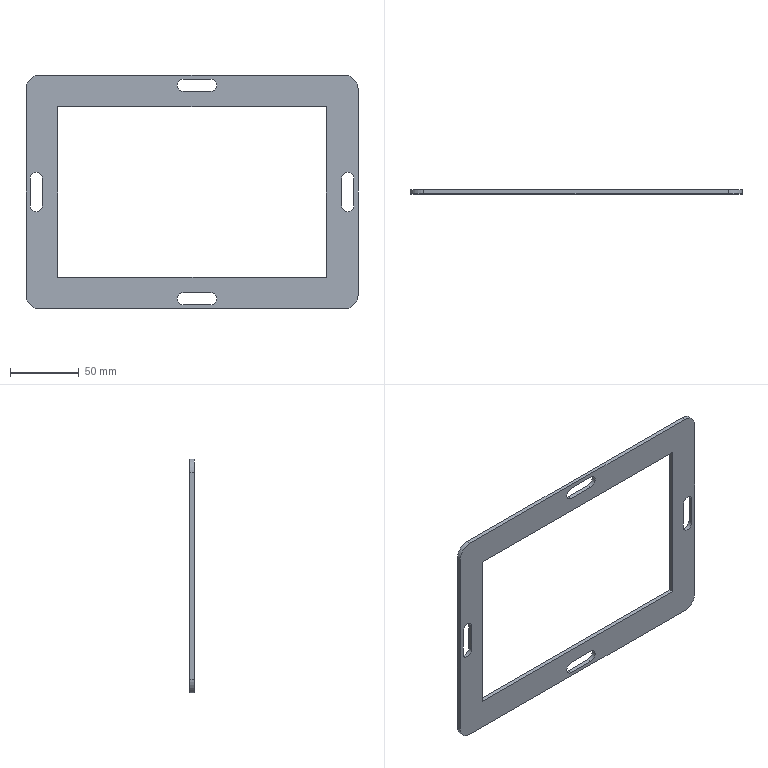Part | STEP file | JBJ-P-1001-02 | 1 solid | 30 faces | box 241.3 x 3 x 170 mm | volume 47230 mm3 | plane 18 | cylinder 12 | commonest cylinder face diameters 9 x8 20 x4
STEP:
#1=CARTESIAN_POINT('',(114.328,3.,3.));
#2=VERTEX_POINT('',#1);
#3=CARTESIAN_POINT('',(114.328,3.,12.));
#4=VERTEX_POINT('',#3);
#5=CARTESIAN_POINT('',(114.328,3.,7.5));
#6=DIRECTION('',(0.,1.,0.));
#7=DIRECTION('',(0.,0.,1.));
#8=AXIS2_PLACEMENT_3D('',#5,#6,#7);
#9=CIRCLE('',#8,4.5);
#10=EDGE_CURVE('',#2,#4,#9,.T.);
#11=ORIENTED_EDGE('',*,*,#10,.F.);
#12=CARTESIAN_POINT('',(134.328,3.,3.));
#13=VERTEX_POINT('',#12);
#14=CARTESIAN_POINT('',(114.328,3.,3.));
#15=DIRECTION('',(-1.,0.,0.));
#16=VECTOR('',#15,1000.);
#17=LINE('',#14,#16);
#18=EDGE_CURVE('',#13,#2,#17,.T.);
#19=ORIENTED_EDGE('',*,*,#18,.F.);
#20=CARTESIAN_POINT('',(134.328,3.,12.));
#21=VERTEX_POINT('',#20);
#22=CARTESIAN_POINT('',(134.328,3.,7.5));
#23=DIRECTION('',(0.,1.,0.));
#24=DIRECTION('',(0.,0.,1.));
#25=AXIS2_PLACEMENT_3D('',#22,#23,#24);
#26=CIRCLE('',#25,4.5);
#27=EDGE_CURVE('',#21,#13,#26,.T.);
#28=ORIENTED_EDGE('',*,*,#27,.F.);
#29=CARTESIAN_POINT('',(134.328,3.,12.));
#30=DIRECTION('',(1.,0.,0.));
#31=VECTOR('',#30,1000.);
#32=LINE('',#29,#31);
#33=EDGE_CURVE('',#4,#21,#32,.T.);
#34=ORIENTED_EDGE('',*,*,#33,.F.);
#35=EDGE_LOOP('',(#11,#19,#28,#34));
#36=FACE_BOUND('',#35,.T.);
#37=CARTESIAN_POINT('',(3.025,3.,95.));
#38=VERTEX_POINT('',#37);
#39=CARTESIAN_POINT('',(12.025,3.,95.));
#40=VERTEX_POINT('',#39);
#41=CARTESIAN_POINT('',(7.525,3.,95.));
#42=DIRECTION('',(0.,1.,0.));
#43=DIRECTION('',(0.,0.,1.));
#44=AXIS2_PLACEMENT_3D('',#41,#42,#43);
#45=CIRCLE('',#44,4.5);
#46=EDGE_CURVE('',#38,#40,#45,.T.);
#47=ORIENTED_EDGE('',*,*,#46,.F.);
#48=CARTESIAN_POINT('',(3.025,3.,75.));
#49=VERTEX_POINT('',#48);
#50=CARTESIAN_POINT('',(3.025,3.,95.));
#51=DIRECTION('',(0.,0.,1.));
#52=VECTOR('',#51,1000.);
#53=LINE('',#50,#52);
#54=EDGE_CURVE('',#49,#38,#53,.T.);
#55=ORIENTED_EDGE('',*,*,#54,.F.);
#56=CARTESIAN_POINT('',(12.025,3.,75.));
#57=VERTEX_POINT('',#56);
#58=CARTESIAN_POINT('',(7.525,3.,75.));
#59=DIRECTION('',(0.,1.,0.));
#60=DIRECTION('',(0.,0.,1.));
#61=AXIS2_PLACEMENT_3D('',#58,#59,#60);
#62=CIRCLE('',#61,4.5);
#63=EDGE_CURVE('',#57,#49,#62,.T.);
#64=ORIENTED_EDGE('',*,*,#63,.F.);
#65=CARTESIAN_POINT('',(12.025,3.,75.));
#66=DIRECTION('',(0.,0.,-1.));
#67=VECTOR('',#66,1000.);
#68=LINE('',#65,#67);
#69=EDGE_CURVE('',#40,#57,#68,.T.);
#70=ORIENTED_EDGE('',*,*,#69,.F.);
#71=EDGE_LOOP('',(#47,#55,#64,#70));
#72=FACE_BOUND('',#71,.T.);
#73=CARTESIAN_POINT('',(114.328,3.,158.));
#74=VERTEX_POINT('',#73);
#75=CARTESIAN_POINT('',(114.328,3.,167.));
#76=VERTEX_POINT('',#75);
#77=CARTESIAN_POINT('',(114.328,3.,162.5));
#78=DIRECTION('',(0.,1.,0.));
#79=DIRECTION('',(0.,0.,1.));
#80=AXIS2_PLACEMENT_3D('',#77,#78,#79);
#81=CIRCLE('',#80,4.5);
#82=EDGE_CURVE('',#74,#76,#81,.T.);
#83=ORIENTED_EDGE('',*,*,#82,.F.);
#84=CARTESIAN_POINT('',(134.328,3.,158.));
#85=VERTEX_POINT('',#84);
#86=CARTESIAN_POINT('',(114.328,3.,158.));
#87=DIRECTION('',(-1.,0.,0.));
#88=VECTOR('',#87,1000.);
#89=LINE('',#86,#88);
#90=EDGE_CURVE('',#85,#74,#89,.T.);
#91=ORIENTED_EDGE('',*,*,#90,.F.);
#92=CARTESIAN_POINT('',(134.328,3.,167.));
#93=VERTEX_POINT('',#92);
#94=CARTESIAN_POINT('',(134.328,3.,162.5));
#95=DIRECTION('',(0.,1.,0.));
#96=DIRECTION('',(0.,0.,1.));
#97=AXIS2_PLACEMENT_3D('',#94,#95,#96);
#98=CIRCLE('',#97,4.5);
#99=EDGE_CURVE('',#93,#85,#98,.T.);
#100=ORIENTED_EDGE('',*,*,#99,.F.);
#101=CARTESIAN_POINT('',(134.328,3.,167.));
#102=DIRECTION('',(1.,0.,0.));
#103=VECTOR('',#102,1000.);
#104=LINE('',#101,#103);
#105=EDGE_CURVE('',#76,#93,#104,.T.);
#106=ORIENTED_EDGE('',*,*,#105,.F.);
#107=EDGE_LOOP('',(#83,#91,#100,#106));
#108=FACE_BOUND('',#107,.T.);
#109=CARTESIAN_POINT('',(229.3,3.,95.));
#110=VERTEX_POINT('',#109);
#111=CARTESIAN_POINT('',(238.3,3.,95.));
#112=VERTEX_POINT('',#111);
#113=CARTESIAN_POINT('',(233.8,3.,95.));
#114=DIRECTION('',(0.,1.,0.));
#115=DIRECTION('',(0.,0.,1.));
#116=AXIS2_PLACEMENT_3D('',#113,#114,#115);
#117=CIRCLE('',#116,4.5);
#118=EDGE_CURVE('',#110,#112,#117,.T.);
#119=ORIENTED_EDGE('',*,*,#118,.F.);
#120=CARTESIAN_POINT('',(229.3,3.,75.));
#121=VERTEX_POINT('',#120);
#122=CARTESIAN_POINT('',(229.3,3.,95.));
#123=DIRECTION('',(0.,0.,1.));
#124=VECTOR('',#123,1000.);
#125=LINE('',#122,#124);
#126=EDGE_CURVE('',#121,#110,#125,.T.);
#127=ORIENTED_EDGE('',*,*,#126,.F.);
#128=CARTESIAN_POINT('',(238.3,3.,75.));
#129=VERTEX_POINT('',#128);
#130=CARTESIAN_POINT('',(233.8,3.,75.));
#131=DIRECTION('',(0.,1.,0.));
#132=DIRECTION('',(0.,0.,1.));
#133=AXIS2_PLACEMENT_3D('',#130,#131,#132);
#134=CIRCLE('',#133,4.5);
#135=EDGE_CURVE('',#129,#121,#134,.T.);
#136=ORIENTED_EDGE('',*,*,#135,.F.);
#137=CARTESIAN_POINT('',(238.3,3.,75.));
#138=DIRECTION('',(0.,0.,-1.));
#139=VECTOR('',#138,1000.);
#140=LINE('',#137,#139);
#141=EDGE_CURVE('',#112,#129,#140,.T.);
#142=ORIENTED_EDGE('',*,*,#141,.F.);
#143=EDGE_LOOP('',(#119,#127,#136,#142));
#144=FACE_BOUND('',#143,.T.);
#145=CARTESIAN_POINT('',(0.,3.,10.));
#146=VERTEX_POINT('',#145);
#147=CARTESIAN_POINT('',(0.,3.,160.));
#148=VERTEX_POINT('',#147);
#149=CARTESIAN_POINT('',(0.,3.,0.));
#150=DIRECTION('',(0.,0.,1.));
#151=VECTOR('',#150,1000.);
#152=LINE('',#149,#151);
#153=EDGE_CURVE('',#146,#148,#152,.T.);
#154=ORIENTED_EDGE('',*,*,#153,.T.);
#155=CARTESIAN_POINT('',(10.,3.,170.));
#156=VERTEX_POINT('',#155);
#157=CARTESIAN_POINT('',(10.,3.,160.));
#158=DIRECTION('',(0.,1.,0.));
#159=DIRECTION('',(0.,0.,1.));
#160=AXIS2_PLACEMENT_3D('',#157,#158,#159);
#161=CIRCLE('',#160,10.);
#162=EDGE_CURVE('',#148,#156,#161,.T.);
#163=ORIENTED_EDGE('',*,*,#162,.T.);
#164=CARTESIAN_POINT('',(231.3,3.,170.));
#165=VERTEX_POINT('',#164);
#166=CARTESIAN_POINT('',(0.,3.,170.));
#167=DIRECTION('',(1.,0.,0.));
#168=VECTOR('',#167,1000.);
#169=LINE('',#166,#168);
#170=EDGE_CURVE('',#156,#165,#169,.T.);
#171=ORIENTED_EDGE('',*,*,#170,.T.);
#172=CARTESIAN_POINT('',(241.3,3.,160.));
#173=VERTEX_POINT('',#172);
#174=CARTESIAN_POINT('',(231.3,3.,160.));
#175=DIRECTION('',(0.,1.,0.));
#176=DIRECTION('',(0.,0.,1.));
#177=AXIS2_PLACEMENT_3D('',#174,#175,#176);
#178=CIRCLE('',#177,10.);
#179=EDGE_CURVE('',#165,#173,#178,.T.);
#180=ORIENTED_EDGE('',*,*,#179,.T.);
#181=CARTESIAN_POINT('',(241.3,3.,10.));
#182=VERTEX_POINT('',#181);
#183=CARTESIAN_POINT('',(241.3,3.,0.));
#184=DIRECTION('',(0.,0.,-1.));
#185=VECTOR('',#184,1000.);
#186=LINE('',#183,#185);
#187=EDGE_CURVE('',#173,#182,#186,.T.);
#188=ORIENTED_EDGE('',*,*,#187,.T.);
#189=CARTESIAN_POINT('',(231.3,3.,0.));
#190=VERTEX_POINT('',#189);
#191=CARTESIAN_POINT('',(231.3,3.,10.));
#192=DIRECTION('',(0.,1.,0.));
#193=DIRECTION('',(0.,0.,1.));
#194=AXIS2_PLACEMENT_3D('',#191,#192,#193);
#195=CIRCLE('',#194,10.);
#196=EDGE_CURVE('',#182,#190,#195,.T.);
#197=ORIENTED_EDGE('',*,*,#196,.T.);
#198=CARTESIAN_POINT('',(10.,3.,0.));
#199=VERTEX_POINT('',#198);
#200=CARTESIAN_POINT('',(0.,3.,0.));
#201=DIRECTION('',(-1.,0.,0.));
#202=VECTOR('',#201,1000.);
#203=LINE('',#200,#202);
#204=EDGE_CURVE('',#190,#199,#203,.T.);
#205=ORIENTED_EDGE('',*,*,#204,.T.);
#206=CARTESIAN_POINT('',(10.,3.,10.));
#207=DIRECTION('',(0.,1.,0.));
#208=DIRECTION('',(0.,0.,1.));
#209=AXIS2_PLACEMENT_3D('',#206,#207,#208);
#210=CIRCLE('',#209,10.);
#211=EDGE_CURVE('',#199,#146,#210,.T.);
#212=ORIENTED_EDGE('',*,*,#211,.T.);
#213=EDGE_LOOP('',(#154,#163,#171,#180,#188,#197,#205,#212));
#214=FACE_OUTER_BOUND('',#213,.T.);
#215=CARTESIAN_POINT('',(23.,3.,147.));
#216=VERTEX_POINT('',#215);
#217=CARTESIAN_POINT('',(218.3,3.,147.));
#218=VERTEX_POINT('',#217);
#219=CARTESIAN_POINT('',(23.,3.,147.));
#220=DIRECTION('',(1.,0.,0.));
#221=VECTOR('',#220,1000.);
#222=LINE('',#219,#221);
#223=EDGE_CURVE('',#216,#218,#222,.T.);
#224=ORIENTED_EDGE('',*,*,#223,.F.);
#225=CARTESIAN_POINT('',(23.,3.,23.));
#226=VERTEX_POINT('',#225);
#227=CARTESIAN_POINT('',(23.,3.,23.));
#228=DIRECTION('',(0.,0.,1.));
#229=VECTOR('',#228,1000.);
#230=LINE('',#227,#229);
#231=EDGE_CURVE('',#226,#216,#230,.T.);
#232=ORIENTED_EDGE('',*,*,#231,.F.);
#233=CARTESIAN_POINT('',(218.3,3.,23.));
#234=VERTEX_POINT('',#233);
#235=CARTESIAN_POINT('',(23.,3.,23.));
#236=DIRECTION('',(-1.,0.,0.));
#237=VECTOR('',#236,1000.);
#238=LINE('',#235,#237);
#239=EDGE_CURVE('',#234,#226,#238,.T.);
#240=ORIENTED_EDGE('',*,*,#239,.F.);
#241=CARTESIAN_POINT('',(218.3,3.,23.));
#242=DIRECTION('',(0.,0.,-1.));
#243=VECTOR('',#242,1000.);
#244=LINE('',#241,#243);
#245=EDGE_CURVE('',#218,#234,#244,.T.);
#246=ORIENTED_EDGE('',*,*,#245,.F.);
#247=EDGE_LOOP('',(#224,#232,#240,#246));
#248=FACE_BOUND('',#247,.T.);
#249=CARTESIAN_POINT('',(0.,3.,0.));
#250=DIRECTION('',(0.,1.,0.));
#251=DIRECTION('',(0.,0.,1.));
#252=AXIS2_PLACEMENT_3D('',#249,#250,#251);
#253=PLANE('',#252);
#254=ADVANCED_FACE('',(#36,#72,#108,#144,#214,#248),#253,.T.);
#255=CARTESIAN_POINT('',(134.328,0.,3.));
#256=VERTEX_POINT('',#255);
#257=CARTESIAN_POINT('',(114.328,0.,3.));
#258=VERTEX_POINT('',#257);
#259=CARTESIAN_POINT('',(0.,0.,3.));
#260=DIRECTION('',(-1.,0.,0.));
#261=VECTOR('',#260,1000.);
#262=LINE('',#259,#261);
#263=EDGE_CURVE('',#256,#258,#262,.T.);
#264=ORIENTED_EDGE('',*,*,#263,.T.);
#265=CARTESIAN_POINT('',(114.328,0.,12.));
#266=VERTEX_POINT('',#265);
#267=CARTESIAN_POINT('',(114.328,0.,7.5));
#268=DIRECTION('',(0.,1.,0.));
#269=DIRECTION('',(0.,0.,1.));
#270=AXIS2_PLACEMENT_3D('',#267,#268,#269);
#271=CIRCLE('',#270,4.5);
#272=EDGE_CURVE('',#258,#266,#271,.T.);
#273=ORIENTED_EDGE('',*,*,#272,.T.);
#274=CARTESIAN_POINT('',(134.328,0.,12.));
#275=VERTEX_POINT('',#274);
#276=CARTESIAN_POINT('',(0.,0.,12.));
#277=DIRECTION('',(1.,0.,0.));
#278=VECTOR('',#277,1000.);
#279=LINE('',#276,#278);
#280=EDGE_CURVE('',#266,#275,#279,.T.);
#281=ORIENTED_EDGE('',*,*,#280,.T.);
#282=CARTESIAN_POINT('',(134.328,0.,7.5));
#283=DIRECTION('',(0.,1.,0.));
#284=DIRECTION('',(0.,0.,1.));
#285=AXIS2_PLACEMENT_3D('',#282,#283,#284);
#286=CIRCLE('',#285,4.5);
#287=EDGE_CURVE('',#275,#256,#286,.T.);
#288=ORIENTED_EDGE('',*,*,#287,.T.);
#289=EDGE_LOOP('',(#264,#273,#281,#288));
#290=FACE_BOUND('',#289,.T.);
#291=CARTESIAN_POINT('',(3.025,0.,75.));
#292=VERTEX_POINT('',#291);
#293=CARTESIAN_POINT('',(3.025,0.,95.));
#294=VERTEX_POINT('',#293);
#295=CARTESIAN_POINT('',(3.025,0.,0.));
#296=DIRECTION('',(0.,0.,1.));
#297=VECTOR('',#296,1000.);
#298=LINE('',#295,#297);
#299=EDGE_CURVE('',#292,#294,#298,.T.);
#300=ORIENTED_EDGE('',*,*,#299,.T.);
#301=CARTESIAN_POINT('',(12.025,0.,95.));
#302=VERTEX_POINT('',#301);
#303=CARTESIAN_POINT('',(7.525,0.,95.));
#304=DIRECTION('',(0.,1.,0.));
#305=DIRECTION('',(0.,0.,1.));
#306=AXIS2_PLACEMENT_3D('',#303,#304,#305);
#307=CIRCLE('',#306,4.5);
#308=EDGE_CURVE('',#294,#302,#307,.T.);
#309=ORIENTED_EDGE('',*,*,#308,.T.);
#310=CARTESIAN_POINT('',(12.025,0.,75.));
#311=VERTEX_POINT('',#310);
#312=CARTESIAN_POINT('',(12.025,0.,0.));
#313=DIRECTION('',(0.,0.,-1.));
#314=VECTOR('',#313,1000.);
#315=LINE('',#312,#314);
#316=EDGE_CURVE('',#302,#311,#315,.T.);
#317=ORIENTED_EDGE('',*,*,#316,.T.);
#318=CARTESIAN_POINT('',(7.525,0.,75.));
#319=DIRECTION('',(0.,1.,0.));
#320=DIRECTION('',(0.,0.,1.));
#321=AXIS2_PLACEMENT_3D('',#318,#319,#320);
#322=CIRCLE('',#321,4.5);
#323=EDGE_CURVE('',#311,#292,#322,.T.);
#324=ORIENTED_EDGE('',*,*,#323,.T.);
#325=EDGE_LOOP('',(#300,#309,#317,#324));
#326=FACE_BOUND('',#325,.T.);
#327=CARTESIAN_POINT('',(134.328,0.,158.));
#328=VERTEX_POINT('',#327);
#329=CARTESIAN_POINT('',(114.328,0.,158.));
#330=VERTEX_POINT('',#329);
#331=CARTESIAN_POINT('',(0.,0.,158.));
#332=DIRECTION('',(-1.,0.,0.));
#333=VECTOR('',#332,1000.);
#334=LINE('',#331,#333);
#335=EDGE_CURVE('',#328,#330,#334,.T.);
#336=ORIENTED_EDGE('',*,*,#335,.T.);
#337=CARTESIAN_POINT('',(114.328,0.,167.));
#338=VERTEX_POINT('',#337);
#339=CARTESIAN_POINT('',(114.328,0.,162.5));
#340=DIRECTION('',(0.,1.,0.));
#341=DIRECTION('',(0.,0.,1.));
#342=AXIS2_PLACEMENT_3D('',#339,#340,#341);
#343=CIRCLE('',#342,4.5);
#344=EDGE_CURVE('',#330,#338,#343,.T.);
#345=ORIENTED_EDGE('',*,*,#344,.T.);
#346=CARTESIAN_POINT('',(134.328,0.,167.));
#347=VERTEX_POINT('',#346);
#348=CARTESIAN_POINT('',(0.,0.,167.));
#349=DIRECTION('',(1.,0.,0.));
#350=VECTOR('',#349,1000.);
#351=LINE('',#348,#350);
#352=EDGE_CURVE('',#338,#347,#351,.T.);
#353=ORIENTED_EDGE('',*,*,#352,.T.);
#354=CARTESIAN_POINT('',(134.328,0.,162.5));
#355=DIRECTION('',(0.,1.,0.));
#356=DIRECTION('',(0.,0.,1.));
#357=AXIS2_PLACEMENT_3D('',#354,#355,#356);
#358=CIRCLE('',#357,4.5);
#359=EDGE_CURVE('',#347,#328,#358,.T.);
#360=ORIENTED_EDGE('',*,*,#359,.T.);
#361=EDGE_LOOP('',(#336,#345,#353,#360));
#362=FACE_BOUND('',#361,.T.);
#363=CARTESIAN_POINT('',(229.3,0.,75.));
#364=VERTEX_POINT('',#363);
#365=CARTESIAN_POINT('',(229.3,0.,95.));
#366=VERTEX_POINT('',#365);
#367=CARTESIAN_POINT('',(229.3,0.,0.));
#368=DIRECTION('',(0.,0.,1.));
#369=VECTOR('',#368,1000.);
#370=LINE('',#367,#369);
#371=EDGE_CURVE('',#364,#366,#370,.T.);
#372=ORIENTED_EDGE('',*,*,#371,.T.);
#373=CARTESIAN_POINT('',(238.3,0.,95.));
#374=VERTEX_POINT('',#373);
#375=CARTESIAN_POINT('',(233.8,0.,95.));
#376=DIRECTION('',(0.,1.,0.));
#377=DIRECTION('',(0.,0.,1.));
#378=AXIS2_PLACEMENT_3D('',#375,#376,#377);
#379=CIRCLE('',#378,4.5);
#380=EDGE_CURVE('',#366,#374,#379,.T.);
#381=ORIENTED_EDGE('',*,*,#380,.T.);
#382=CARTESIAN_POINT('',(238.3,0.,75.));
#383=VERTEX_POINT('',#382);
#384=CARTESIAN_POINT('',(238.3,0.,0.));
#385=DIRECTION('',(0.,0.,-1.));
#386=VECTOR('',#385,1000.);
#387=LINE('',#384,#386);
#388=EDGE_CURVE('',#374,#383,#387,.T.);
#389=ORIENTED_EDGE('',*,*,#388,.T.);
#390=CARTESIAN_POINT('',(233.8,0.,75.));
#391=DIRECTION('',(0.,1.,0.));
#392=DIRECTION('',(0.,0.,1.));
#393=AXIS2_PLACEMENT_3D('',#390,#391,#392);
#394=CIRCLE('',#393,4.5);
#395=EDGE_CURVE('',#383,#364,#394,.T.);
#396=ORIENTED_EDGE('',*,*,#395,.T.);
#397=EDGE_LOOP('',(#372,#381,#389,#396));
#398=FACE_BOUND('',#397,.T.);
#399=CARTESIAN_POINT('',(10.,0.,170.));
#400=VERTEX_POINT('',#399);
#401=CARTESIAN_POINT('',(231.3,0.,170.));
#402=VERTEX_POINT('',#401);
#403=CARTESIAN_POINT('',(0.,0.,170.));
#404=DIRECTION('',(1.,0.,0.));
#405=VECTOR('',#404,1000.);
#406=LINE('',#403,#405);
#407=EDGE_CURVE('',#400,#402,#406,.T.);
#408=ORIENTED_EDGE('',*,*,#407,.F.);
#409=CARTESIAN_POINT('',(0.,0.,160.));
#410=VERTEX_POINT('',#409);
#411=CARTESIAN_POINT('',(10.,0.,160.));
#412=DIRECTION('',(0.,-1.,0.));
#413=DIRECTION('',(0.,0.,1.));
#414=AXIS2_PLACEMENT_3D('',#411,#412,#413);
#415=CIRCLE('',#414,10.);
#416=EDGE_CURVE('',#400,#410,#415,.T.);
#417=ORIENTED_EDGE('',*,*,#416,.T.);
#418=CARTESIAN_POINT('',(0.,0.,10.));
#419=VERTEX_POINT('',#418);
#420=CARTESIAN_POINT('',(0.,0.,0.));
#421=DIRECTION('',(0.,0.,1.));
#422=VECTOR('',#421,1000.);
#423=LINE('',#420,#422);
#424=EDGE_CURVE('',#419,#410,#423,.T.);
#425=ORIENTED_EDGE('',*,*,#424,.F.);
#426=CARTESIAN_POINT('',(10.,0.,0.));
#427=VERTEX_POINT('',#426);
#428=CARTESIAN_POINT('',(10.,0.,10.));
#429=DIRECTION('',(0.,-1.,0.));
#430=DIRECTION('',(0.,0.,1.));
#431=AXIS2_PLACEMENT_3D('',#428,#429,#430);
#432=CIRCLE('',#431,10.);
#433=EDGE_CURVE('',#419,#427,#432,.T.);
#434=ORIENTED_EDGE('',*,*,#433,.T.);
#435=CARTESIAN_POINT('',(231.3,0.,0.));
#436=VERTEX_POINT('',#435);
#437=CARTESIAN_POINT('',(0.,0.,0.));
#438=DIRECTION('',(-1.,0.,0.));
#439=VECTOR('',#438,1000.);
#440=LINE('',#437,#439);
#441=EDGE_CURVE('',#436,#427,#440,.T.);
#442=ORIENTED_EDGE('',*,*,#441,.F.);
#443=CARTESIAN_POINT('',(241.3,0.,10.));
#444=VERTEX_POINT('',#443);
#445=CARTESIAN_POINT('',(231.3,0.,10.));
#446=DIRECTION('',(0.,-1.,0.));
#447=DIRECTION('',(0.,0.,1.));
#448=AXIS2_PLACEMENT_3D('',#445,#446,#447);
#449=CIRCLE('',#448,10.);
#450=EDGE_CURVE('',#436,#444,#449,.T.);
#451=ORIENTED_EDGE('',*,*,#450,.T.);
#452=CARTESIAN_POINT('',(241.3,0.,160.));
#453=VERTEX_POINT('',#452);
#454=CARTESIAN_POINT('',(241.3,0.,0.));
#455=DIRECTION('',(0.,0.,-1.));
#456=VECTOR('',#455,1000.);
#457=LINE('',#454,#456);
#458=EDGE_CURVE('',#453,#444,#457,.T.);
#459=ORIENTED_EDGE('',*,*,#458,.F.);
#460=CARTESIAN_POINT('',(231.3,0.,160.));
#461=DIRECTION('',(0.,-1.,0.));
#462=DIRECTION('',(0.,0.,1.));
#463=AXIS2_PLACEMENT_3D('',#460,#461,#462);
#464=CIRCLE('',#463,10.);
#465=EDGE_CURVE('',#453,#402,#464,.T.);
#466=ORIENTED_EDGE('',*,*,#465,.T.);
#467=EDGE_LOOP('',(#408,#417,#425,#434,#442,#451,#459,#466));
#468=FACE_OUTER_BOUND('',#467,.T.);
#469=CARTESIAN_POINT('',(23.,0.,23.));
#470=VERTEX_POINT('',#469);
#471=CARTESIAN_POINT('',(23.,0.,147.));
#472=VERTEX_POINT('',#471);
#473=CARTESIAN_POINT('',(23.,0.,23.));
#474=DIRECTION('',(0.,0.,1.));
#475=VECTOR('',#474,1000.);
#476=LINE('',#473,#475);
#477=EDGE_CURVE('',#470,#472,#476,.T.);
#478=ORIENTED_EDGE('',*,*,#477,.T.);
#479=CARTESIAN_POINT('',(218.3,0.,147.));
#480=VERTEX_POINT('',#479);
#481=CARTESIAN_POINT('',(23.,0.,147.));
#482=DIRECTION('',(1.,0.,0.));
#483=VECTOR('',#482,1000.);
#484=LINE('',#481,#483);
#485=EDGE_CURVE('',#472,#480,#484,.T.);
#486=ORIENTED_EDGE('',*,*,#485,.T.);
#487=CARTESIAN_POINT('',(218.3,0.,23.));
#488=VERTEX_POINT('',#487);
#489=CARTESIAN_POINT('',(218.3,0.,23.));
#490=DIRECTION('',(0.,0.,-1.));
#491=VECTOR('',#490,1000.);
#492=LINE('',#489,#491);
#493=EDGE_CURVE('',#480,#488,#492,.T.);
#494=ORIENTED_EDGE('',*,*,#493,.T.);
#495=CARTESIAN_POINT('',(23.,0.,23.));
#496=DIRECTION('',(-1.,0.,0.));
#497=VECTOR('',#496,1000.);
#498=LINE('',#495,#497);
#499=EDGE_CURVE('',#488,#470,#498,.T.);
#500=ORIENTED_EDGE('',*,*,#499,.T.);
#501=EDGE_LOOP('',(#478,#486,#494,#500));
#502=FACE_BOUND('',#501,.T.);
#503=CARTESIAN_POINT('',(0.,0.,0.));
#504=DIRECTION('',(0.,1.,0.));
#505=DIRECTION('',(0.,0.,1.));
#506=AXIS2_PLACEMENT_3D('',#503,#504,#505);
#507=PLANE('',#506);
#508=ADVANCED_FACE('',(#290,#326,#362,#398,#468,#502),#507,.F.);
#509=ORIENTED_EDGE('',*,*,#424,.T.);
#510=CARTESIAN_POINT('',(0.,3.,160.));
#511=DIRECTION('',(0.,1.,0.));
#512=VECTOR('',#511,1000.);
#513=LINE('',#510,#512);
#514=EDGE_CURVE('',#410,#148,#513,.T.);
#515=ORIENTED_EDGE('',*,*,#514,.T.);
#516=ORIENTED_EDGE('',*,*,#153,.F.);
#517=CARTESIAN_POINT('',(0.,3.,10.));
#518=DIRECTION('',(0.,-1.,0.));
#519=VECTOR('',#518,1000.);
#520=LINE('',#517,#519);
#521=EDGE_CURVE('',#146,#419,#520,.T.);
#522=ORIENTED_EDGE('',*,*,#521,.T.);
#523=EDGE_LOOP('',(#509,#515,#516,#522));
#524=FACE_OUTER_BOUND('',#523,.T.);
#525=CARTESIAN_POINT('',(0.,3.,0.));
#526=DIRECTION('',(1.,0.,0.));
#527=DIRECTION('',(0.,0.,-1.));
#528=AXIS2_PLACEMENT_3D('',#525,#526,#527);
#529=PLANE('',#528);
#530=ADVANCED_FACE('',(#524),#529,.F.);
#531=ORIENTED_EDGE('',*,*,#170,.F.);
#532=CARTESIAN_POINT('',(10.,3.,170.));
#533=DIRECTION('',(0.,-1.,0.));
#534=VECTOR('',#533,1000.);
#535=LINE('',#532,#534);
#536=EDGE_CURVE('',#156,#400,#535,.T.);
#537=ORIENTED_EDGE('',*,*,#536,.T.);
#538=ORIENTED_EDGE('',*,*,#407,.T.);
#539=CARTESIAN_POINT('',(231.3,3.,170.));
#540=DIRECTION('',(0.,1.,0.));
#541=VECTOR('',#540,1000.);
#542=LINE('',#539,#541);
#543=EDGE_CURVE('',#402,#165,#542,.T.);
#544=ORIENTED_EDGE('',*,*,#543,.T.);
#545=EDGE_LOOP('',(#531,#537,#538,#544));
#546=FACE_OUTER_BOUND('',#545,.T.);
#547=CARTESIAN_POINT('',(0.,3.,170.));
#548=DIRECTION('',(0.,0.,-1.));
#549=DIRECTION('',(-1.,0.,0.));
#550=AXIS2_PLACEMENT_3D('',#547,#548,#549);
#551=PLANE('',#550);
#552=ADVANCED_FACE('',(#546),#551,.F.);
#553=ORIENTED_EDGE('',*,*,#187,.F.);
#554=CARTESIAN_POINT('',(241.3,3.,160.));
#555=DIRECTION('',(0.,-1.,0.));
#556=VECTOR('',#555,1000.);
#557=LINE('',#554,#556);
#558=EDGE_CURVE('',#173,#453,#557,.T.);
#559=ORIENTED_EDGE('',*,*,#558,.T.);
#560=ORIENTED_EDGE('',*,*,#458,.T.);
#561=CARTESIAN_POINT('',(241.3,3.,10.));
#562=DIRECTION('',(0.,1.,0.));
#563=VECTOR('',#562,1000.);
#564=LINE('',#561,#563);
#565=EDGE_CURVE('',#444,#182,#564,.T.);
#566=ORIENTED_EDGE('',*,*,#565,.T.);
#567=EDGE_LOOP('',(#553,#559,#560,#566));
#568=FACE_OUTER_BOUND('',#567,.T.);
#569=CARTESIAN_POINT('',(241.3,3.,0.));
#570=DIRECTION('',(-1.,0.,0.));
#571=DIRECTION('',(0.,0.,1.));
#572=AXIS2_PLACEMENT_3D('',#569,#570,#571);
#573=PLANE('',#572);
#574=ADVANCED_FACE('',(#568),#573,.F.);
#575=ORIENTED_EDGE('',*,*,#204,.F.);
#576=CARTESIAN_POINT('',(231.3,3.,0.));
#577=DIRECTION('',(0.,-1.,0.));
#578=VECTOR('',#577,1000.);
#579=LINE('',#576,#578);
#580=EDGE_CURVE('',#190,#436,#579,.T.);
#581=ORIENTED_EDGE('',*,*,#580,.T.);
#582=ORIENTED_EDGE('',*,*,#441,.T.);
#583=CARTESIAN_POINT('',(10.,3.,0.));
#584=DIRECTION('',(0.,1.,0.));
#585=VECTOR('',#584,1000.);
#586=LINE('',#583,#585);
#587=EDGE_CURVE('',#427,#199,#586,.T.);
#588=ORIENTED_EDGE('',*,*,#587,.T.);
#589=EDGE_LOOP('',(#575,#581,#582,#588));
#590=FACE_OUTER_BOUND('',#589,.T.);
#591=CARTESIAN_POINT('',(0.,3.,0.));
#592=DIRECTION('',(0.,0.,1.));
#593=DIRECTION('',(1.,0.,0.));
#594=AXIS2_PLACEMENT_3D('',#591,#592,#593);
#595=PLANE('',#594);
#596=ADVANCED_FACE('',(#590),#595,.F.);
#597=ORIENTED_EDGE('',*,*,#477,.F.);
#598=CARTESIAN_POINT('',(23.,3.,23.));
#599=DIRECTION('',(0.,-1.,0.));
#600=VECTOR('',#599,1000.);
#601=LINE('',#598,#600);
#602=EDGE_CURVE('',#226,#470,#601,.T.);
#603=ORIENTED_EDGE('',*,*,#602,.F.);
#604=ORIENTED_EDGE('',*,*,#231,.T.);
#605=CARTESIAN_POINT('',(23.,3.,147.));
#606=DIRECTION('',(0.,-1.,0.));
#607=VECTOR('',#606,1000.);
#608=LINE('',#605,#607);
#609=EDGE_CURVE('',#216,#472,#608,.T.);
#610=ORIENTED_EDGE('',*,*,#609,.T.);
#611=EDGE_LOOP('',(#597,#603,#604,#610));
#612=FACE_OUTER_BOUND('',#611,.T.);
#613=CARTESIAN_POINT('',(23.,3.,23.));
#614=DIRECTION('',(1.,0.,0.));
#615=DIRECTION('',(0.,0.,-1.));
#616=AXIS2_PLACEMENT_3D('',#613,#614,#615);
#617=PLANE('',#616);
#618=ADVANCED_FACE('',(#612),#617,.T.);
#619=ORIENTED_EDGE('',*,*,#485,.F.);
#620=ORIENTED_EDGE('',*,*,#609,.F.);
#621=ORIENTED_EDGE('',*,*,#223,.T.);
#622=CARTESIAN_POINT('',(218.3,3.,147.));
#623=DIRECTION('',(0.,-1.,0.));
#624=VECTOR('',#623,1000.);
#625=LINE('',#622,#624);
#626=EDGE_CURVE('',#218,#480,#625,.T.);
#627=ORIENTED_EDGE('',*,*,#626,.T.);
#628=EDGE_LOOP('',(#619,#620,#621,#627));
#629=FACE_OUTER_BOUND('',#628,.T.);
#630=CARTESIAN_POINT('',(23.,3.,147.));
#631=DIRECTION('',(0.,0.,-1.));
#632=DIRECTION('',(-1.,0.,0.));
#633=AXIS2_PLACEMENT_3D('',#630,#631,#632);
#634=PLANE('',#633);
#635=ADVANCED_FACE('',(#629),#634,.T.);
#636=ORIENTED_EDGE('',*,*,#493,.F.);
#637=ORIENTED_EDGE('',*,*,#626,.F.);
#638=ORIENTED_EDGE('',*,*,#245,.T.);
#639=CARTESIAN_POINT('',(218.3,3.,23.));
#640=DIRECTION('',(0.,-1.,0.));
#641=VECTOR('',#640,1000.);
#642=LINE('',#639,#641);
#643=EDGE_CURVE('',#234,#488,#642,.T.);
#644=ORIENTED_EDGE('',*,*,#643,.T.);
#645=EDGE_LOOP('',(#636,#637,#638,#644));
#646=FACE_OUTER_BOUND('',#645,.T.);
#647=CARTESIAN_POINT('',(218.3,3.,23.));
#648=DIRECTION('',(-1.,0.,0.));
#649=DIRECTION('',(0.,0.,1.));
#650=AXIS2_PLACEMENT_3D('',#647,#648,#649);
#651=PLANE('',#650);
#652=ADVANCED_FACE('',(#646),#651,.T.);
#653=ORIENTED_EDGE('',*,*,#499,.F.);
#654=ORIENTED_EDGE('',*,*,#643,.F.);
#655=ORIENTED_EDGE('',*,*,#239,.T.);
#656=ORIENTED_EDGE('',*,*,#602,.T.);
#657=EDGE_LOOP('',(#653,#654,#655,#656));
#658=FACE_OUTER_BOUND('',#657,.T.);
#659=CARTESIAN_POINT('',(23.,3.,23.));
#660=DIRECTION('',(0.,0.,1.));
#661=DIRECTION('',(1.,0.,0.));
#662=AXIS2_PLACEMENT_3D('',#659,#660,#661);
#663=PLANE('',#662);
#664=ADVANCED_FACE('',(#658),#663,.T.);
#665=ORIENTED_EDGE('',*,*,#162,.F.);
#666=ORIENTED_EDGE('',*,*,#514,.F.);
#667=ORIENTED_EDGE('',*,*,#416,.F.);
#668=ORIENTED_EDGE('',*,*,#536,.F.);
#669=EDGE_LOOP('',(#665,#666,#667,#668));
#670=FACE_OUTER_BOUND('',#669,.T.);
#671=CARTESIAN_POINT('',(10.,3.,160.));
#672=DIRECTION('',(0.,-1.,0.));
#673=DIRECTION('',(0.,0.,-1.));
#674=AXIS2_PLACEMENT_3D('',#671,#672,#673);
#675=CYLINDRICAL_SURFACE('',#674,10.);
#676=ADVANCED_FACE('',(#670),#675,.T.);
#677=ORIENTED_EDGE('',*,*,#179,.F.);
#678=ORIENTED_EDGE('',*,*,#543,.F.);
#679=ORIENTED_EDGE('',*,*,#465,.F.);
#680=ORIENTED_EDGE('',*,*,#558,.F.);
#681=EDGE_LOOP('',(#677,#678,#679,#680));
#682=FACE_OUTER_BOUND('',#681,.T.);
#683=CARTESIAN_POINT('',(231.3,3.,160.));
#684=DIRECTION('',(0.,-1.,0.));
#685=DIRECTION('',(0.,0.,-1.));
#686=AXIS2_PLACEMENT_3D('',#683,#684,#685);
#687=CYLINDRICAL_SURFACE('',#686,10.);
#688=ADVANCED_FACE('',(#682),#687,.T.);
#689=ORIENTED_EDGE('',*,*,#196,.F.);
#690=ORIENTED_EDGE('',*,*,#565,.F.);
#691=ORIENTED_EDGE('',*,*,#450,.F.);
#692=ORIENTED_EDGE('',*,*,#580,.F.);
#693=EDGE_LOOP('',(#689,#690,#691,#692));
#694=FACE_OUTER_BOUND('',#693,.T.);
#695=CARTESIAN_POINT('',(231.3,3.,10.));
#696=DIRECTION('',(0.,-1.,0.));
#697=DIRECTION('',(0.,0.,-1.));
#698=AXIS2_PLACEMENT_3D('',#695,#696,#697);
#699=CYLINDRICAL_SURFACE('',#698,10.);
#700=ADVANCED_FACE('',(#694),#699,.T.);
#701=ORIENTED_EDGE('',*,*,#211,.F.);
#702=ORIENTED_EDGE('',*,*,#587,.F.);
#703=ORIENTED_EDGE('',*,*,#433,.F.);
#704=ORIENTED_EDGE('',*,*,#521,.F.);
#705=EDGE_LOOP('',(#701,#702,#703,#704));
#706=FACE_OUTER_BOUND('',#705,.T.);
#707=CARTESIAN_POINT('',(10.,3.,10.));
#708=DIRECTION('',(0.,-1.,0.));
#709=DIRECTION('',(0.,0.,-1.));
#710=AXIS2_PLACEMENT_3D('',#707,#708,#709);
#711=CYLINDRICAL_SURFACE('',#710,10.);
#712=ADVANCED_FACE('',(#706),#711,.T.);
#713=CARTESIAN_POINT('',(229.3,-7.,95.));
#714=DIRECTION('',(0.,1.,0.));
#715=VECTOR('',#714,1000.);
#716=LINE('',#713,#715);
#717=EDGE_CURVE('',#366,#110,#716,.T.);
#718=ORIENTED_EDGE('',*,*,#717,.T.);
#719=ORIENTED_EDGE('',*,*,#118,.T.);
#720=CARTESIAN_POINT('',(238.3,-7.,95.));
#721=DIRECTION('',(0.,1.,0.));
#722=VECTOR('',#721,1000.);
#723=LINE('',#720,#722);
#724=EDGE_CURVE('',#374,#112,#723,.T.);
#725=ORIENTED_EDGE('',*,*,#724,.F.);
#726=ORIENTED_EDGE('',*,*,#380,.F.);
#727=EDGE_LOOP('',(#718,#719,#725,#726));
#728=FACE_OUTER_BOUND('',#727,.T.);
#729=CARTESIAN_POINT('',(233.8,-7.,95.));
#730=DIRECTION('',(0.,1.,0.));
#731=DIRECTION('',(0.,0.,1.));
#732=AXIS2_PLACEMENT_3D('',#729,#730,#731);
#733=CYLINDRICAL_SURFACE('',#732,4.5);
#734=ADVANCED_FACE('',(#728),#733,.F.);
#735=CARTESIAN_POINT('',(229.3,-7.,75.));
#736=DIRECTION('',(0.,1.,0.));
#737=VECTOR('',#736,1000.);
#738=LINE('',#735,#737);
#739=EDGE_CURVE('',#364,#121,#738,.T.);
#740=ORIENTED_EDGE('',*,*,#739,.T.);
#741=ORIENTED_EDGE('',*,*,#126,.T.);
#742=ORIENTED_EDGE('',*,*,#717,.F.);
#743=ORIENTED_EDGE('',*,*,#371,.F.);
#744=EDGE_LOOP('',(#740,#741,#742,#743));
#745=FACE_OUTER_BOUND('',#744,.T.);
#746=CARTESIAN_POINT('',(229.3,-7.,95.));
#747=DIRECTION('',(-1.,0.,0.));
#748=DIRECTION('',(0.,0.,1.));
#749=AXIS2_PLACEMENT_3D('',#746,#747,#748);
#750=PLANE('',#749);
#751=ADVANCED_FACE('',(#745),#750,.F.);
#752=CARTESIAN_POINT('',(238.3,-7.,75.));
#753=DIRECTION('',(0.,1.,0.));
#754=VECTOR('',#753,1000.);
#755=LINE('',#752,#754);
#756=EDGE_CURVE('',#383,#129,#755,.T.);
#757=ORIENTED_EDGE('',*,*,#756,.T.);
#758=ORIENTED_EDGE('',*,*,#135,.T.);
#759=ORIENTED_EDGE('',*,*,#739,.F.);
#760=ORIENTED_EDGE('',*,*,#395,.F.);
#761=EDGE_LOOP('',(#757,#758,#759,#760));
#762=FACE_OUTER_BOUND('',#761,.T.);
#763=CARTESIAN_POINT('',(233.8,-7.,75.));
#764=DIRECTION('',(0.,1.,0.));
#765=DIRECTION('',(0.,0.,1.));
#766=AXIS2_PLACEMENT_3D('',#763,#764,#765);
#767=CYLINDRICAL_SURFACE('',#766,4.5);
#768=ADVANCED_FACE('',(#762),#767,.F.);
#769=ORIENTED_EDGE('',*,*,#724,.T.);
#770=ORIENTED_EDGE('',*,*,#141,.T.);
#771=ORIENTED_EDGE('',*,*,#756,.F.);
#772=ORIENTED_EDGE('',*,*,#388,.F.);
#773=EDGE_LOOP('',(#769,#770,#771,#772));
#774=FACE_OUTER_BOUND('',#773,.T.);
#775=CARTESIAN_POINT('',(238.3,-7.,75.));
#776=DIRECTION('',(1.,0.,0.));
#777=DIRECTION('',(0.,0.,-1.));
#778=AXIS2_PLACEMENT_3D('',#775,#776,#777);
#779=PLANE('',#778);
#780=ADVANCED_FACE('',(#774),#779,.F.);
#781=CARTESIAN_POINT('',(114.328,-7.,158.));
#782=DIRECTION('',(0.,1.,0.));
#783=VECTOR('',#782,1000.);
#784=LINE('',#781,#783);
#785=EDGE_CURVE('',#330,#74,#784,.T.);
#786=ORIENTED_EDGE('',*,*,#785,.T.);
#787=ORIENTED_EDGE('',*,*,#82,.T.);
#788=CARTESIAN_POINT('',(114.328,-7.,167.));
#789=DIRECTION('',(0.,1.,0.));
#790=VECTOR('',#789,1000.);
#791=LINE('',#788,#790);
#792=EDGE_CURVE('',#338,#76,#791,.T.);
#793=ORIENTED_EDGE('',*,*,#792,.F.);
#794=ORIENTED_EDGE('',*,*,#344,.F.);
#795=EDGE_LOOP('',(#786,#787,#793,#794));
#796=FACE_OUTER_BOUND('',#795,.T.);
#797=CARTESIAN_POINT('',(114.328,-7.,162.5));
#798=DIRECTION('',(0.,1.,0.));
#799=DIRECTION('',(0.,0.,1.));
#800=AXIS2_PLACEMENT_3D('',#797,#798,#799);
#801=CYLINDRICAL_SURFACE('',#800,4.5);
#802=ADVANCED_FACE('',(#796),#801,.F.);
#803=CARTESIAN_POINT('',(134.328,-7.,158.));
#804=DIRECTION('',(0.,1.,0.));
#805=VECTOR('',#804,1000.);
#806=LINE('',#803,#805);
#807=EDGE_CURVE('',#328,#85,#806,.T.);
#808=ORIENTED_EDGE('',*,*,#807,.T.);
#809=ORIENTED_EDGE('',*,*,#90,.T.);
#810=ORIENTED_EDGE('',*,*,#785,.F.);
#811=ORIENTED_EDGE('',*,*,#335,.F.);
#812=EDGE_LOOP('',(#808,#809,#810,#811));
#813=FACE_OUTER_BOUND('',#812,.T.);
#814=CARTESIAN_POINT('',(114.328,-7.,158.));
#815=DIRECTION('',(0.,0.,-1.));
#816=DIRECTION('',(-1.,0.,0.));
#817=AXIS2_PLACEMENT_3D('',#814,#815,#816);
#818=PLANE('',#817);
#819=ADVANCED_FACE('',(#813),#818,.F.);
#820=CARTESIAN_POINT('',(134.328,-7.,167.));
#821=DIRECTION('',(0.,1.,0.));
#822=VECTOR('',#821,1000.);
#823=LINE('',#820,#822);
#824=EDGE_CURVE('',#347,#93,#823,.T.);
#825=ORIENTED_EDGE('',*,*,#824,.T.);
#826=ORIENTED_EDGE('',*,*,#99,.T.);
#827=ORIENTED_EDGE('',*,*,#807,.F.);
#828=ORIENTED_EDGE('',*,*,#359,.F.);
#829=EDGE_LOOP('',(#825,#826,#827,#828));
#830=FACE_OUTER_BOUND('',#829,.T.);
#831=CARTESIAN_POINT('',(134.328,-7.,162.5));
#832=DIRECTION('',(0.,1.,0.));
#833=DIRECTION('',(0.,0.,1.));
#834=AXIS2_PLACEMENT_3D('',#831,#832,#833);
#835=CYLINDRICAL_SURFACE('',#834,4.5);
#836=ADVANCED_FACE('',(#830),#835,.F.);
#837=ORIENTED_EDGE('',*,*,#792,.T.);
#838=ORIENTED_EDGE('',*,*,#105,.T.);
#839=ORIENTED_EDGE('',*,*,#824,.F.);
#840=ORIENTED_EDGE('',*,*,#352,.F.);
#841=EDGE_LOOP('',(#837,#838,#839,#840));
#842=FACE_OUTER_BOUND('',#841,.T.);
#843=CARTESIAN_POINT('',(134.328,-7.,167.));
#844=DIRECTION('',(0.,0.,1.));
#845=DIRECTION('',(1.,0.,0.));
#846=AXIS2_PLACEMENT_3D('',#843,#844,#845);
#847=PLANE('',#846);
#848=ADVANCED_FACE('',(#842),#847,.F.);
#849=CARTESIAN_POINT('',(3.025,-7.,95.));
#850=DIRECTION('',(0.,1.,0.));
#851=VECTOR('',#850,1000.);
#852=LINE('',#849,#851);
#853=EDGE_CURVE('',#294,#38,#852,.T.);
#854=ORIENTED_EDGE('',*,*,#853,.T.);
#855=ORIENTED_EDGE('',*,*,#46,.T.);
#856=CARTESIAN_POINT('',(12.025,-7.,95.));
#857=DIRECTION('',(0.,1.,0.));
#858=VECTOR('',#857,1000.);
#859=LINE('',#856,#858);
#860=EDGE_CURVE('',#302,#40,#859,.T.);
#861=ORIENTED_EDGE('',*,*,#860,.F.);
#862=ORIENTED_EDGE('',*,*,#308,.F.);
#863=EDGE_LOOP('',(#854,#855,#861,#862));
#864=FACE_OUTER_BOUND('',#863,.T.);
#865=CARTESIAN_POINT('',(7.525,-7.,95.));
#866=DIRECTION('',(0.,1.,0.));
#867=DIRECTION('',(0.,0.,1.));
#868=AXIS2_PLACEMENT_3D('',#865,#866,#867);
#869=CYLINDRICAL_SURFACE('',#868,4.5);
#870=ADVANCED_FACE('',(#864),#869,.F.);
#871=CARTESIAN_POINT('',(3.025,-7.,75.));
#872=DIRECTION('',(0.,1.,0.));
#873=VECTOR('',#872,1000.);
#874=LINE('',#871,#873);
#875=EDGE_CURVE('',#292,#49,#874,.T.);
#876=ORIENTED_EDGE('',*,*,#875,.T.);
#877=ORIENTED_EDGE('',*,*,#54,.T.);
#878=ORIENTED_EDGE('',*,*,#853,.F.);
#879=ORIENTED_EDGE('',*,*,#299,.F.);
#880=EDGE_LOOP('',(#876,#877,#878,#879));
#881=FACE_OUTER_BOUND('',#880,.T.);
#882=CARTESIAN_POINT('',(3.025,-7.,95.));
#883=DIRECTION('',(-1.,0.,0.));
#884=DIRECTION('',(0.,0.,1.));
#885=AXIS2_PLACEMENT_3D('',#882,#883,#884);
#886=PLANE('',#885);
#887=ADVANCED_FACE('',(#881),#886,.F.);
#888=CARTESIAN_POINT('',(12.025,-7.,75.));
#889=DIRECTION('',(0.,1.,0.));
#890=VECTOR('',#889,1000.);
#891=LINE('',#888,#890);
#892=EDGE_CURVE('',#311,#57,#891,.T.);
#893=ORIENTED_EDGE('',*,*,#892,.T.);
#894=ORIENTED_EDGE('',*,*,#63,.T.);
#895=ORIENTED_EDGE('',*,*,#875,.F.);
#896=ORIENTED_EDGE('',*,*,#323,.F.);
#897=EDGE_LOOP('',(#893,#894,#895,#896));
#898=FACE_OUTER_BOUND('',#897,.T.);
#899=CARTESIAN_POINT('',(7.525,-7.,75.));
#900=DIRECTION('',(0.,1.,0.));
#901=DIRECTION('',(0.,0.,1.));
#902=AXIS2_PLACEMENT_3D('',#899,#900,#901);
#903=CYLINDRICAL_SURFACE('',#902,4.5);
#904=ADVANCED_FACE('',(#898),#903,.F.);
#905=ORIENTED_EDGE('',*,*,#860,.T.);
#906=ORIENTED_EDGE('',*,*,#69,.T.);
#907=ORIENTED_EDGE('',*,*,#892,.F.);
#908=ORIENTED_EDGE('',*,*,#316,.F.);
#909=EDGE_LOOP('',(#905,#906,#907,#908));
#910=FACE_OUTER_BOUND('',#909,.T.);
#911=CARTESIAN_POINT('',(12.025,-7.,75.));
#912=DIRECTION('',(1.,0.,0.));
#913=DIRECTION('',(0.,0.,-1.));
#914=AXIS2_PLACEMENT_3D('',#911,#912,#913);
#915=PLANE('',#914);
#916=ADVANCED_FACE('',(#910),#915,.F.);
#917=CARTESIAN_POINT('',(114.328,-7.,3.));
#918=DIRECTION('',(0.,1.,0.));
#919=VECTOR('',#918,1000.);
#920=LINE('',#917,#919);
#921=EDGE_CURVE('',#258,#2,#920,.T.);
#922=ORIENTED_EDGE('',*,*,#921,.T.);
#923=ORIENTED_EDGE('',*,*,#10,.T.);
#924=CARTESIAN_POINT('',(114.328,-7.,12.));
#925=DIRECTION('',(0.,1.,0.));
#926=VECTOR('',#925,1000.);
#927=LINE('',#924,#926);
#928=EDGE_CURVE('',#266,#4,#927,.T.);
#929=ORIENTED_EDGE('',*,*,#928,.F.);
#930=ORIENTED_EDGE('',*,*,#272,.F.);
#931=EDGE_LOOP('',(#922,#923,#929,#930));
#932=FACE_OUTER_BOUND('',#931,.T.);
#933=CARTESIAN_POINT('',(114.328,-7.,7.5));
#934=DIRECTION('',(0.,1.,0.));
#935=DIRECTION('',(0.,0.,1.));
#936=AXIS2_PLACEMENT_3D('',#933,#934,#935);
#937=CYLINDRICAL_SURFACE('',#936,4.5);
#938=ADVANCED_FACE('',(#932),#937,.F.);
#939=CARTESIAN_POINT('',(134.328,-7.,3.));
#940=DIRECTION('',(0.,1.,0.));
#941=VECTOR('',#940,1000.);
#942=LINE('',#939,#941);
#943=EDGE_CURVE('',#256,#13,#942,.T.);
#944=ORIENTED_EDGE('',*,*,#943,.T.);
#945=ORIENTED_EDGE('',*,*,#18,.T.);
#946=ORIENTED_EDGE('',*,*,#921,.F.);
#947=ORIENTED_EDGE('',*,*,#263,.F.);
#948=EDGE_LOOP('',(#944,#945,#946,#947));
#949=FACE_OUTER_BOUND('',#948,.T.);
#950=CARTESIAN_POINT('',(114.328,-7.,3.));
#951=DIRECTION('',(0.,0.,-1.));
#952=DIRECTION('',(-1.,0.,0.));
#953=AXIS2_PLACEMENT_3D('',#950,#951,#952);
#954=PLANE('',#953);
#955=ADVANCED_FACE('',(#949),#954,.F.);
#956=CARTESIAN_POINT('',(134.328,-7.,12.));
#957=DIRECTION('',(0.,1.,0.));
#958=VECTOR('',#957,1000.);
#959=LINE('',#956,#958);
#960=EDGE_CURVE('',#275,#21,#959,.T.);
#961=ORIENTED_EDGE('',*,*,#960,.T.);
#962=ORIENTED_EDGE('',*,*,#27,.T.);
#963=ORIENTED_EDGE('',*,*,#943,.F.);
#964=ORIENTED_EDGE('',*,*,#287,.F.);
#965=EDGE_LOOP('',(#961,#962,#963,#964));
#966=FACE_OUTER_BOUND('',#965,.T.);
#967=CARTESIAN_POINT('',(134.328,-7.,7.5));
#968=DIRECTION('',(0.,1.,0.));
#969=DIRECTION('',(0.,0.,1.));
#970=AXIS2_PLACEMENT_3D('',#967,#968,#969);
#971=CYLINDRICAL_SURFACE('',#970,4.5);
#972=ADVANCED_FACE('',(#966),#971,.F.);
#973=ORIENTED_EDGE('',*,*,#928,.T.);
#974=ORIENTED_EDGE('',*,*,#33,.T.);
#975=ORIENTED_EDGE('',*,*,#960,.F.);
#976=ORIENTED_EDGE('',*,*,#280,.F.);
#977=EDGE_LOOP('',(#973,#974,#975,#976));
#978=FACE_OUTER_BOUND('',#977,.T.);
#979=CARTESIAN_POINT('',(134.328,-7.,12.));
#980=DIRECTION('',(0.,0.,1.));
#981=DIRECTION('',(1.,0.,0.));
#982=AXIS2_PLACEMENT_3D('',#979,#980,#981);
#983=PLANE('',#982);
#984=ADVANCED_FACE('',(#978),#983,.F.);
#985=CLOSED_SHELL('',(#254,#508,#530,#552,#574,#596,#618,#635,#652,#664,#676,#688,#700,#712,#734,#751,#768,#780,#802,#819,#836,#848,#870,#887,#904,#916,#938,#955,#972,#984));
#986=MANIFOLD_SOLID_BREP('',#985);
#987=CARTESIAN_POINT('',(0.,0.,0.));
#988=DIRECTION('',(0.,0.,1.));
#989=DIRECTION('',(1.,0.,0.));
#990=AXIS2_PLACEMENT_3D('',#987,#988,#989);
#991=(LENGTH_UNIT()NAMED_UNIT(*)SI_UNIT(.MILLI.,.METRE.));
#992=UNCERTAINTY_MEASURE_WITH_UNIT(LENGTH_MEASURE(0.00001),#991,'','');
#993=(NAMED_UNIT(*)PLANE_ANGLE_UNIT()SI_UNIT($,.RADIAN.));
#994=(NAMED_UNIT(*)SI_UNIT($,.STERADIAN.)SOLID_ANGLE_UNIT());
#995=(GEOMETRIC_REPRESENTATION_CONTEXT(3)GLOBAL_UNCERTAINTY_ASSIGNED_CONTEXT((#992))GLOBAL_UNIT_ASSIGNED_CONTEXT((#991,#993,#994))REPRESENTATION_CONTEXT('',''));
#996=ADVANCED_BREP_SHAPE_REPRESENTATION('',(#986,#990),#995);